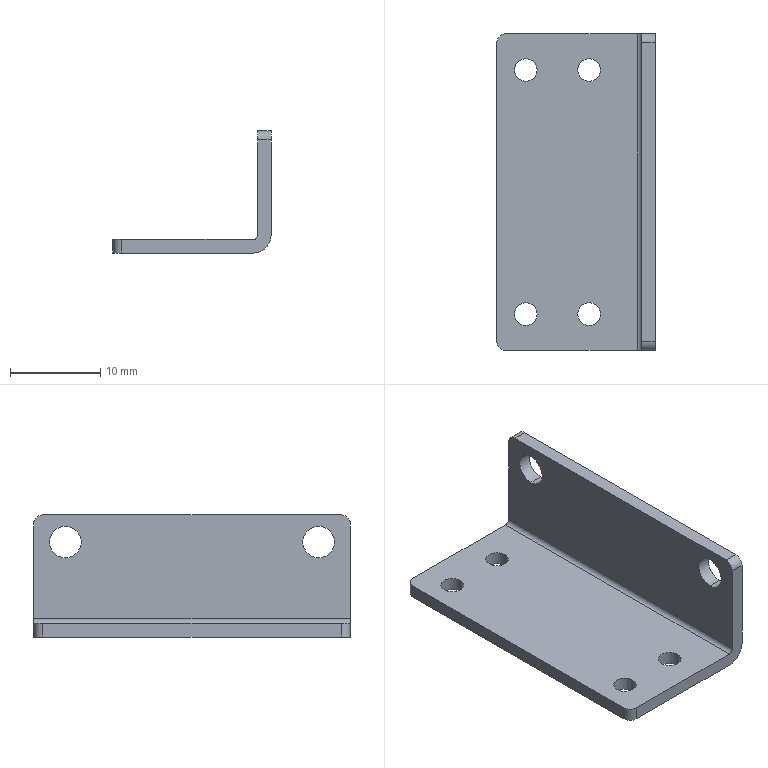Part | SolidWorks | features BaseBody 1 | 1 solid | 26 faces | box 17.5 x 35 x 13.5 mm | volume 1461 mm3 | cylinder 18 | plane 8 | commonest cylinder face diameters 2.5 x8 2 x4 3.5 x4 1 x1 4 x1
STEP:
#1=CARTESIAN_POINT('',(296.997,233.806,-401.845));
#2=VERTEX_POINT('',#1);
#3=CARTESIAN_POINT('',(294.497,233.806,-401.845));
#4=VERTEX_POINT('',#3);
#5=CARTESIAN_POINT('',(295.747,233.806,-401.845));
#6=DIRECTION('',(0.,0.,-1.));
#7=DIRECTION('',(-1.,0.,0.));
#8=AXIS2_PLACEMENT_3D('',#5,#6,#7);
#9=CIRCLE('',#8,1.25);
#10=EDGE_CURVE('',#2,#4,#9,.T.);
#11=ORIENTED_EDGE('',*,*,#10,.F.);
#12=CARTESIAN_POINT('',(296.997,233.806,-403.345));
#13=VERTEX_POINT('',#12);
#14=CARTESIAN_POINT('',(296.997,233.806,-94.345));
#15=DIRECTION('',(0.,0.,-1.));
#16=VECTOR('',#15,1000.);
#17=LINE('',#14,#16);
#18=EDGE_CURVE('',#2,#13,#17,.T.);
#19=ORIENTED_EDGE('',*,*,#18,.T.);
#20=CARTESIAN_POINT('',(294.497,233.806,-403.345));
#21=VERTEX_POINT('',#20);
#22=CARTESIAN_POINT('',(295.747,233.806,-403.345));
#23=DIRECTION('',(0.,0.,-1.));
#24=DIRECTION('',(-1.,0.,0.));
#25=AXIS2_PLACEMENT_3D('',#22,#23,#24);
#26=CIRCLE('',#25,1.25);
#27=EDGE_CURVE('',#13,#21,#26,.T.);
#28=ORIENTED_EDGE('',*,*,#27,.T.);
#29=CARTESIAN_POINT('',(294.497,233.806,-94.345));
#30=DIRECTION('',(0.,0.,-1.));
#31=VECTOR('',#30,1000.);
#32=LINE('',#29,#31);
#33=EDGE_CURVE('',#4,#21,#32,.T.);
#34=ORIENTED_EDGE('',*,*,#33,.F.);
#35=EDGE_LOOP('',(#11,#19,#28,#34));
#36=FACE_OUTER_BOUND('',#35,.T.);
#37=CARTESIAN_POINT('',(295.747,233.806,-94.345));
#38=DIRECTION('',(0.,0.,-1.));
#39=DIRECTION('',(-1.,0.,0.));
#40=AXIS2_PLACEMENT_3D('',#37,#38,#39);
#41=CYLINDRICAL_SURFACE('',#40,1.25);
#42=ADVANCED_FACE('',(#36),#41,.F.);
#43=CARTESIAN_POINT('',(296.997,206.806,-401.845));
#44=VERTEX_POINT('',#43);
#45=CARTESIAN_POINT('',(294.497,206.806,-401.845));
#46=VERTEX_POINT('',#45);
#47=CARTESIAN_POINT('',(295.747,206.806,-401.845));
#48=DIRECTION('',(0.,0.,-1.));
#49=DIRECTION('',(-1.,0.,0.));
#50=AXIS2_PLACEMENT_3D('',#47,#48,#49);
#51=CIRCLE('',#50,1.25);
#52=EDGE_CURVE('',#44,#46,#51,.T.);
#53=ORIENTED_EDGE('',*,*,#52,.F.);
#54=CARTESIAN_POINT('',(296.997,206.806,-403.345));
#55=VERTEX_POINT('',#54);
#56=CARTESIAN_POINT('',(296.997,206.806,-94.345));
#57=DIRECTION('',(0.,0.,-1.));
#58=VECTOR('',#57,1000.);
#59=LINE('',#56,#58);
#60=EDGE_CURVE('',#44,#55,#59,.T.);
#61=ORIENTED_EDGE('',*,*,#60,.T.);
#62=CARTESIAN_POINT('',(294.497,206.806,-403.345));
#63=VERTEX_POINT('',#62);
#64=CARTESIAN_POINT('',(295.747,206.806,-403.345));
#65=DIRECTION('',(0.,0.,-1.));
#66=DIRECTION('',(-1.,0.,0.));
#67=AXIS2_PLACEMENT_3D('',#64,#65,#66);
#68=CIRCLE('',#67,1.25);
#69=EDGE_CURVE('',#55,#63,#68,.T.);
#70=ORIENTED_EDGE('',*,*,#69,.T.);
#71=CARTESIAN_POINT('',(294.497,206.806,-94.345));
#72=DIRECTION('',(0.,0.,-1.));
#73=VECTOR('',#72,1000.);
#74=LINE('',#71,#73);
#75=EDGE_CURVE('',#46,#63,#74,.T.);
#76=ORIENTED_EDGE('',*,*,#75,.F.);
#77=EDGE_LOOP('',(#53,#61,#70,#76));
#78=FACE_OUTER_BOUND('',#77,.T.);
#79=CARTESIAN_POINT('',(295.747,206.806,-94.345));
#80=DIRECTION('',(0.,0.,-1.));
#81=DIRECTION('',(-1.,0.,0.));
#82=AXIS2_PLACEMENT_3D('',#79,#80,#81);
#83=CYLINDRICAL_SURFACE('',#82,1.25);
#84=ADVANCED_FACE('',(#78),#83,.F.);
#85=CARTESIAN_POINT('',(303.997,233.806,-401.845));
#86=VERTEX_POINT('',#85);
#87=CARTESIAN_POINT('',(301.497,233.806,-401.845));
#88=VERTEX_POINT('',#87);
#89=CARTESIAN_POINT('',(302.747,233.806,-401.845));
#90=DIRECTION('',(0.,0.,-1.));
#91=DIRECTION('',(-1.,0.,0.));
#92=AXIS2_PLACEMENT_3D('',#89,#90,#91);
#93=CIRCLE('',#92,1.25);
#94=EDGE_CURVE('',#86,#88,#93,.T.);
#95=ORIENTED_EDGE('',*,*,#94,.F.);
#96=CARTESIAN_POINT('',(303.997,233.806,-403.345));
#97=VERTEX_POINT('',#96);
#98=CARTESIAN_POINT('',(303.997,233.806,-94.345));
#99=DIRECTION('',(0.,0.,-1.));
#100=VECTOR('',#99,1000.);
#101=LINE('',#98,#100);
#102=EDGE_CURVE('',#86,#97,#101,.T.);
#103=ORIENTED_EDGE('',*,*,#102,.T.);
#104=CARTESIAN_POINT('',(301.497,233.806,-403.345));
#105=VERTEX_POINT('',#104);
#106=CARTESIAN_POINT('',(302.747,233.806,-403.345));
#107=DIRECTION('',(0.,0.,-1.));
#108=DIRECTION('',(-1.,0.,0.));
#109=AXIS2_PLACEMENT_3D('',#106,#107,#108);
#110=CIRCLE('',#109,1.25);
#111=EDGE_CURVE('',#97,#105,#110,.T.);
#112=ORIENTED_EDGE('',*,*,#111,.T.);
#113=CARTESIAN_POINT('',(301.497,233.806,-94.345));
#114=DIRECTION('',(0.,0.,-1.));
#115=VECTOR('',#114,1000.);
#116=LINE('',#113,#115);
#117=EDGE_CURVE('',#88,#105,#116,.T.);
#118=ORIENTED_EDGE('',*,*,#117,.F.);
#119=EDGE_LOOP('',(#95,#103,#112,#118));
#120=FACE_OUTER_BOUND('',#119,.T.);
#121=CARTESIAN_POINT('',(302.747,233.806,-94.345));
#122=DIRECTION('',(0.,0.,-1.));
#123=DIRECTION('',(-1.,0.,0.));
#124=AXIS2_PLACEMENT_3D('',#121,#122,#123);
#125=CYLINDRICAL_SURFACE('',#124,1.25);
#126=ADVANCED_FACE('',(#120),#125,.F.);
#127=CARTESIAN_POINT('',(303.997,206.806,-401.845));
#128=VERTEX_POINT('',#127);
#129=CARTESIAN_POINT('',(301.497,206.806,-401.845));
#130=VERTEX_POINT('',#129);
#131=CARTESIAN_POINT('',(302.747,206.806,-401.845));
#132=DIRECTION('',(0.,0.,-1.));
#133=DIRECTION('',(-1.,0.,0.));
#134=AXIS2_PLACEMENT_3D('',#131,#132,#133);
#135=CIRCLE('',#134,1.25);
#136=EDGE_CURVE('',#128,#130,#135,.T.);
#137=ORIENTED_EDGE('',*,*,#136,.F.);
#138=CARTESIAN_POINT('',(303.997,206.806,-403.345));
#139=VERTEX_POINT('',#138);
#140=CARTESIAN_POINT('',(303.997,206.806,-94.345));
#141=DIRECTION('',(0.,0.,-1.));
#142=VECTOR('',#141,1000.);
#143=LINE('',#140,#142);
#144=EDGE_CURVE('',#128,#139,#143,.T.);
#145=ORIENTED_EDGE('',*,*,#144,.T.);
#146=CARTESIAN_POINT('',(301.497,206.806,-403.345));
#147=VERTEX_POINT('',#146);
#148=CARTESIAN_POINT('',(302.747,206.806,-403.345));
#149=DIRECTION('',(0.,0.,-1.));
#150=DIRECTION('',(-1.,0.,0.));
#151=AXIS2_PLACEMENT_3D('',#148,#149,#150);
#152=CIRCLE('',#151,1.25);
#153=EDGE_CURVE('',#139,#147,#152,.T.);
#154=ORIENTED_EDGE('',*,*,#153,.T.);
#155=CARTESIAN_POINT('',(301.497,206.806,-94.345));
#156=DIRECTION('',(0.,0.,-1.));
#157=VECTOR('',#156,1000.);
#158=LINE('',#155,#157);
#159=EDGE_CURVE('',#130,#147,#158,.T.);
#160=ORIENTED_EDGE('',*,*,#159,.F.);
#161=EDGE_LOOP('',(#137,#145,#154,#160));
#162=FACE_OUTER_BOUND('',#161,.T.);
#163=CARTESIAN_POINT('',(302.747,206.806,-94.345));
#164=DIRECTION('',(0.,0.,-1.));
#165=DIRECTION('',(-1.,0.,0.));
#166=AXIS2_PLACEMENT_3D('',#163,#164,#165);
#167=CYLINDRICAL_SURFACE('',#166,1.25);
#168=ADVANCED_FACE('',(#162),#167,.F.);
#169=CARTESIAN_POINT('',(308.547,234.306,-394.595));
#170=VERTEX_POINT('',#169);
#171=CARTESIAN_POINT('',(308.547,234.306,-391.095));
#172=VERTEX_POINT('',#171);
#173=CARTESIAN_POINT('',(308.547,234.306,-392.845));
#174=DIRECTION('',(-1.,0.,0.));
#175=DIRECTION('',(0.,0.,-1.));
#176=AXIS2_PLACEMENT_3D('',#173,#174,#175);
#177=CIRCLE('',#176,1.75);
#178=EDGE_CURVE('',#170,#172,#177,.T.);
#179=ORIENTED_EDGE('',*,*,#178,.T.);
#180=CARTESIAN_POINT('',(310.047,234.306,-391.095));
#181=VERTEX_POINT('',#180);
#182=CARTESIAN_POINT('',(7.247,234.306,-391.095));
#183=DIRECTION('',(1.,0.,0.));
#184=VECTOR('',#183,1000.);
#185=LINE('',#182,#184);
#186=EDGE_CURVE('',#172,#181,#185,.T.);
#187=ORIENTED_EDGE('',*,*,#186,.T.);
#188=CARTESIAN_POINT('',(310.047,234.306,-394.595));
#189=VERTEX_POINT('',#188);
#190=CARTESIAN_POINT('',(310.047,234.306,-392.845));
#191=DIRECTION('',(1.,0.,0.));
#192=DIRECTION('',(0.,0.,-1.));
#193=AXIS2_PLACEMENT_3D('',#190,#191,#192);
#194=CIRCLE('',#193,1.75);
#195=EDGE_CURVE('',#181,#189,#194,.T.);
#196=ORIENTED_EDGE('',*,*,#195,.T.);
#197=CARTESIAN_POINT('',(7.247,234.306,-394.595));
#198=DIRECTION('',(1.,0.,0.));
#199=VECTOR('',#198,1000.);
#200=LINE('',#197,#199);
#201=EDGE_CURVE('',#170,#189,#200,.T.);
#202=ORIENTED_EDGE('',*,*,#201,.F.);
#203=EDGE_LOOP('',(#179,#187,#196,#202));
#204=FACE_OUTER_BOUND('',#203,.T.);
#205=CARTESIAN_POINT('',(7.247,234.306,-392.845));
#206=DIRECTION('',(1.,0.,0.));
#207=DIRECTION('',(0.,0.,-1.));
#208=AXIS2_PLACEMENT_3D('',#205,#206,#207);
#209=CYLINDRICAL_SURFACE('',#208,1.75);
#210=ADVANCED_FACE('',(#204),#209,.F.);
#211=CARTESIAN_POINT('',(308.547,206.306,-394.595));
#212=VERTEX_POINT('',#211);
#213=CARTESIAN_POINT('',(308.547,206.306,-391.095));
#214=VERTEX_POINT('',#213);
#215=CARTESIAN_POINT('',(308.547,206.306,-392.845));
#216=DIRECTION('',(-1.,0.,0.));
#217=DIRECTION('',(0.,0.,-1.));
#218=AXIS2_PLACEMENT_3D('',#215,#216,#217);
#219=CIRCLE('',#218,1.75);
#220=EDGE_CURVE('',#212,#214,#219,.T.);
#221=ORIENTED_EDGE('',*,*,#220,.T.);
#222=CARTESIAN_POINT('',(310.047,206.306,-391.095));
#223=VERTEX_POINT('',#222);
#224=CARTESIAN_POINT('',(7.247,206.306,-391.095));
#225=DIRECTION('',(1.,0.,0.));
#226=VECTOR('',#225,1000.);
#227=LINE('',#224,#226);
#228=EDGE_CURVE('',#214,#223,#227,.T.);
#229=ORIENTED_EDGE('',*,*,#228,.T.);
#230=CARTESIAN_POINT('',(310.047,206.306,-394.595));
#231=VERTEX_POINT('',#230);
#232=CARTESIAN_POINT('',(310.047,206.306,-392.845));
#233=DIRECTION('',(1.,0.,0.));
#234=DIRECTION('',(0.,0.,-1.));
#235=AXIS2_PLACEMENT_3D('',#232,#233,#234);
#236=CIRCLE('',#235,1.75);
#237=EDGE_CURVE('',#223,#231,#236,.T.);
#238=ORIENTED_EDGE('',*,*,#237,.T.);
#239=CARTESIAN_POINT('',(7.247,206.306,-394.595));
#240=DIRECTION('',(1.,0.,0.));
#241=VECTOR('',#240,1000.);
#242=LINE('',#239,#241);
#243=EDGE_CURVE('',#212,#231,#242,.T.);
#244=ORIENTED_EDGE('',*,*,#243,.F.);
#245=EDGE_LOOP('',(#221,#229,#238,#244));
#246=FACE_OUTER_BOUND('',#245,.T.);
#247=CARTESIAN_POINT('',(7.247,206.306,-392.845));
#248=DIRECTION('',(1.,0.,0.));
#249=DIRECTION('',(0.,0.,-1.));
#250=AXIS2_PLACEMENT_3D('',#247,#248,#249);
#251=CYLINDRICAL_SURFACE('',#250,1.75);
#252=ADVANCED_FACE('',(#246),#251,.F.);
#253=CARTESIAN_POINT('',(295.747,233.806,-403.345));
#254=DIRECTION('',(0.,0.,-1.));
#255=DIRECTION('',(-1.,0.,0.));
#256=AXIS2_PLACEMENT_3D('',#253,#254,#255);
#257=CIRCLE('',#256,1.25);
#258=EDGE_CURVE('',#21,#13,#257,.T.);
#259=ORIENTED_EDGE('',*,*,#258,.F.);
#260=ORIENTED_EDGE('',*,*,#27,.F.);
#261=EDGE_LOOP('',(#259,#260));
#262=FACE_BOUND('',#261,.T.);
#263=CARTESIAN_POINT('',(295.747,206.806,-403.345));
#264=DIRECTION('',(0.,0.,-1.));
#265=DIRECTION('',(-1.,0.,0.));
#266=AXIS2_PLACEMENT_3D('',#263,#264,#265);
#267=CIRCLE('',#266,1.25);
#268=EDGE_CURVE('',#63,#55,#267,.T.);
#269=ORIENTED_EDGE('',*,*,#268,.F.);
#270=ORIENTED_EDGE('',*,*,#69,.F.);
#271=EDGE_LOOP('',(#269,#270));
#272=FACE_BOUND('',#271,.T.);
#273=CARTESIAN_POINT('',(302.747,233.806,-403.345));
#274=DIRECTION('',(0.,0.,-1.));
#275=DIRECTION('',(-1.,0.,0.));
#276=AXIS2_PLACEMENT_3D('',#273,#274,#275);
#277=CIRCLE('',#276,1.25);
#278=EDGE_CURVE('',#105,#97,#277,.T.);
#279=ORIENTED_EDGE('',*,*,#278,.F.);
#280=ORIENTED_EDGE('',*,*,#111,.F.);
#281=EDGE_LOOP('',(#279,#280));
#282=FACE_BOUND('',#281,.T.);
#283=CARTESIAN_POINT('',(302.747,206.806,-403.345));
#284=DIRECTION('',(0.,0.,-1.));
#285=DIRECTION('',(-1.,0.,0.));
#286=AXIS2_PLACEMENT_3D('',#283,#284,#285);
#287=CIRCLE('',#286,1.25);
#288=EDGE_CURVE('',#147,#139,#287,.T.);
#289=ORIENTED_EDGE('',*,*,#288,.F.);
#290=ORIENTED_EDGE('',*,*,#153,.F.);
#291=EDGE_LOOP('',(#289,#290));
#292=FACE_BOUND('',#291,.T.);
#293=CARTESIAN_POINT('',(292.547,236.806,-403.345));
#294=VERTEX_POINT('',#293);
#295=CARTESIAN_POINT('',(292.547,203.806,-403.345));
#296=VERTEX_POINT('',#295);
#297=CARTESIAN_POINT('',(292.547,237.806,-403.345));
#298=DIRECTION('',(0.,-1.,0.));
#299=VECTOR('',#298,1000.);
#300=LINE('',#297,#299);
#301=EDGE_CURVE('',#294,#296,#300,.T.);
#302=ORIENTED_EDGE('',*,*,#301,.F.);
#303=CARTESIAN_POINT('',(293.547,237.806,-403.345));
#304=VERTEX_POINT('',#303);
#305=CARTESIAN_POINT('',(293.547,236.806,-403.345));
#306=DIRECTION('',(0.,0.,1.));
#307=DIRECTION('',(-1.,0.,0.));
#308=AXIS2_PLACEMENT_3D('',#305,#306,#307);
#309=CIRCLE('',#308,1.);
#310=EDGE_CURVE('',#304,#294,#309,.T.);
#311=ORIENTED_EDGE('',*,*,#310,.F.);
#312=CARTESIAN_POINT('',(308.047,237.806,-403.345));
#313=VERTEX_POINT('',#312);
#314=CARTESIAN_POINT('',(308.047,237.806,-403.345));
#315=DIRECTION('',(-1.,0.,0.));
#316=VECTOR('',#315,1000.);
#317=LINE('',#314,#316);
#318=EDGE_CURVE('',#313,#304,#317,.T.);
#319=ORIENTED_EDGE('',*,*,#318,.F.);
#320=CARTESIAN_POINT('',(308.047,202.806,-403.345));
#321=VERTEX_POINT('',#320);
#322=CARTESIAN_POINT('',(308.047,237.806,-403.345));
#323=DIRECTION('',(0.,1.,0.));
#324=VECTOR('',#323,1000.);
#325=LINE('',#322,#324);
#326=EDGE_CURVE('',#321,#313,#325,.T.);
#327=ORIENTED_EDGE('',*,*,#326,.F.);
#328=CARTESIAN_POINT('',(293.547,202.806,-403.345));
#329=VERTEX_POINT('',#328);
#330=CARTESIAN_POINT('',(308.047,202.806,-403.345));
#331=DIRECTION('',(1.,0.,0.));
#332=VECTOR('',#331,1000.);
#333=LINE('',#330,#332);
#334=EDGE_CURVE('',#329,#321,#333,.T.);
#335=ORIENTED_EDGE('',*,*,#334,.F.);
#336=CARTESIAN_POINT('',(293.547,203.806,-403.345));
#337=DIRECTION('',(0.,0.,1.));
#338=DIRECTION('',(1.,0.,0.));
#339=AXIS2_PLACEMENT_3D('',#336,#337,#338);
#340=CIRCLE('',#339,1.);
#341=EDGE_CURVE('',#296,#329,#340,.T.);
#342=ORIENTED_EDGE('',*,*,#341,.F.);
#343=EDGE_LOOP('',(#302,#311,#319,#327,#335,#342));
#344=FACE_OUTER_BOUND('',#343,.T.);
#345=CARTESIAN_POINT('',(308.047,237.806,-403.345));
#346=DIRECTION('',(0.,0.,1.));
#347=DIRECTION('',(1.,0.,0.));
#348=AXIS2_PLACEMENT_3D('',#345,#346,#347);
#349=PLANE('',#348);
#350=ADVANCED_FACE('',(#262,#272,#282,#292,#344),#349,.F.);
#351=ORIENTED_EDGE('',*,*,#18,.F.);
#352=CARTESIAN_POINT('',(295.747,233.806,-401.845));
#353=DIRECTION('',(0.,0.,-1.));
#354=DIRECTION('',(-1.,0.,0.));
#355=AXIS2_PLACEMENT_3D('',#352,#353,#354);
#356=CIRCLE('',#355,1.25);
#357=EDGE_CURVE('',#4,#2,#356,.T.);
#358=ORIENTED_EDGE('',*,*,#357,.F.);
#359=ORIENTED_EDGE('',*,*,#33,.T.);
#360=ORIENTED_EDGE('',*,*,#258,.T.);
#361=EDGE_LOOP('',(#351,#358,#359,#360));
#362=FACE_OUTER_BOUND('',#361,.T.);
#363=CARTESIAN_POINT('',(295.747,233.806,-94.345));
#364=DIRECTION('',(0.,0.,-1.));
#365=DIRECTION('',(-1.,0.,0.));
#366=AXIS2_PLACEMENT_3D('',#363,#364,#365);
#367=CYLINDRICAL_SURFACE('',#366,1.25);
#368=ADVANCED_FACE('',(#362),#367,.F.);
#369=ORIENTED_EDGE('',*,*,#60,.F.);
#370=CARTESIAN_POINT('',(295.747,206.806,-401.845));
#371=DIRECTION('',(0.,0.,-1.));
#372=DIRECTION('',(-1.,0.,0.));
#373=AXIS2_PLACEMENT_3D('',#370,#371,#372);
#374=CIRCLE('',#373,1.25);
#375=EDGE_CURVE('',#46,#44,#374,.T.);
#376=ORIENTED_EDGE('',*,*,#375,.F.);
#377=ORIENTED_EDGE('',*,*,#75,.T.);
#378=ORIENTED_EDGE('',*,*,#268,.T.);
#379=EDGE_LOOP('',(#369,#376,#377,#378));
#380=FACE_OUTER_BOUND('',#379,.T.);
#381=CARTESIAN_POINT('',(295.747,206.806,-94.345));
#382=DIRECTION('',(0.,0.,-1.));
#383=DIRECTION('',(-1.,0.,0.));
#384=AXIS2_PLACEMENT_3D('',#381,#382,#383);
#385=CYLINDRICAL_SURFACE('',#384,1.25);
#386=ADVANCED_FACE('',(#380),#385,.F.);
#387=ORIENTED_EDGE('',*,*,#102,.F.);
#388=CARTESIAN_POINT('',(302.747,233.806,-401.845));
#389=DIRECTION('',(0.,0.,-1.));
#390=DIRECTION('',(-1.,0.,0.));
#391=AXIS2_PLACEMENT_3D('',#388,#389,#390);
#392=CIRCLE('',#391,1.25);
#393=EDGE_CURVE('',#88,#86,#392,.T.);
#394=ORIENTED_EDGE('',*,*,#393,.F.);
#395=ORIENTED_EDGE('',*,*,#117,.T.);
#396=ORIENTED_EDGE('',*,*,#278,.T.);
#397=EDGE_LOOP('',(#387,#394,#395,#396));
#398=FACE_OUTER_BOUND('',#397,.T.);
#399=CARTESIAN_POINT('',(302.747,233.806,-94.345));
#400=DIRECTION('',(0.,0.,-1.));
#401=DIRECTION('',(-1.,0.,0.));
#402=AXIS2_PLACEMENT_3D('',#399,#400,#401);
#403=CYLINDRICAL_SURFACE('',#402,1.25);
#404=ADVANCED_FACE('',(#398),#403,.F.);
#405=ORIENTED_EDGE('',*,*,#144,.F.);
#406=CARTESIAN_POINT('',(302.747,206.806,-401.845));
#407=DIRECTION('',(0.,0.,-1.));
#408=DIRECTION('',(-1.,0.,0.));
#409=AXIS2_PLACEMENT_3D('',#406,#407,#408);
#410=CIRCLE('',#409,1.25);
#411=EDGE_CURVE('',#130,#128,#410,.T.);
#412=ORIENTED_EDGE('',*,*,#411,.F.);
#413=ORIENTED_EDGE('',*,*,#159,.T.);
#414=ORIENTED_EDGE('',*,*,#288,.T.);
#415=EDGE_LOOP('',(#405,#412,#413,#414));
#416=FACE_OUTER_BOUND('',#415,.T.);
#417=CARTESIAN_POINT('',(302.747,206.806,-94.345));
#418=DIRECTION('',(0.,0.,-1.));
#419=DIRECTION('',(-1.,0.,0.));
#420=AXIS2_PLACEMENT_3D('',#417,#418,#419);
#421=CYLINDRICAL_SURFACE('',#420,1.25);
#422=ADVANCED_FACE('',(#416),#421,.F.);
#423=CARTESIAN_POINT('',(292.547,203.806,-401.845));
#424=VERTEX_POINT('',#423);
#425=CARTESIAN_POINT('',(292.547,203.806,-403.345));
#426=DIRECTION('',(0.,0.,-1.));
#427=VECTOR('',#426,1000.);
#428=LINE('',#425,#427);
#429=EDGE_CURVE('',#424,#296,#428,.T.);
#430=ORIENTED_EDGE('',*,*,#429,.T.);
#431=ORIENTED_EDGE('',*,*,#341,.T.);
#432=CARTESIAN_POINT('',(293.547,202.806,-401.845));
#433=VERTEX_POINT('',#432);
#434=CARTESIAN_POINT('',(293.547,202.806,-403.345));
#435=DIRECTION('',(0.,0.,1.));
#436=VECTOR('',#435,1000.);
#437=LINE('',#434,#436);
#438=EDGE_CURVE('',#329,#433,#437,.T.);
#439=ORIENTED_EDGE('',*,*,#438,.T.);
#440=CARTESIAN_POINT('',(293.547,203.806,-401.845));
#441=DIRECTION('',(0.,0.,-1.));
#442=DIRECTION('',(1.,0.,0.));
#443=AXIS2_PLACEMENT_3D('',#440,#441,#442);
#444=CIRCLE('',#443,1.);
#445=EDGE_CURVE('',#433,#424,#444,.T.);
#446=ORIENTED_EDGE('',*,*,#445,.T.);
#447=EDGE_LOOP('',(#430,#431,#439,#446));
#448=FACE_OUTER_BOUND('',#447,.T.);
#449=CARTESIAN_POINT('',(293.547,203.806,-403.345));
#450=DIRECTION('',(0.,0.,1.));
#451=DIRECTION('',(1.,0.,0.));
#452=AXIS2_PLACEMENT_3D('',#449,#450,#451);
#453=CYLINDRICAL_SURFACE('',#452,1.);
#454=ADVANCED_FACE('',(#448),#453,.T.);
#455=CARTESIAN_POINT('',(292.547,236.806,-401.845));
#456=VERTEX_POINT('',#455);
#457=CARTESIAN_POINT('',(292.547,237.806,-401.845));
#458=DIRECTION('',(0.,-1.,0.));
#459=VECTOR('',#458,1000.);
#460=LINE('',#457,#459);
#461=EDGE_CURVE('',#456,#424,#460,.T.);
#462=ORIENTED_EDGE('',*,*,#461,.F.);
#463=CARTESIAN_POINT('',(292.547,236.806,-403.345));
#464=DIRECTION('',(0.,0.,1.));
#465=VECTOR('',#464,1000.);
#466=LINE('',#463,#465);
#467=EDGE_CURVE('',#294,#456,#466,.T.);
#468=ORIENTED_EDGE('',*,*,#467,.F.);
#469=ORIENTED_EDGE('',*,*,#301,.T.);
#470=ORIENTED_EDGE('',*,*,#429,.F.);
#471=EDGE_LOOP('',(#462,#468,#469,#470));
#472=FACE_OUTER_BOUND('',#471,.T.);
#473=CARTESIAN_POINT('',(292.547,237.806,-403.345));
#474=DIRECTION('',(1.,0.,0.));
#475=DIRECTION('',(0.,0.,-1.));
#476=AXIS2_PLACEMENT_3D('',#473,#474,#475);
#477=PLANE('',#476);
#478=ADVANCED_FACE('',(#472),#477,.F.);
#479=CARTESIAN_POINT('',(293.547,237.806,-401.845));
#480=VERTEX_POINT('',#479);
#481=CARTESIAN_POINT('',(293.547,237.806,-401.345));
#482=DIRECTION('',(0.,0.,-1.));
#483=VECTOR('',#482,1000.);
#484=LINE('',#481,#483);
#485=EDGE_CURVE('',#480,#304,#484,.T.);
#486=ORIENTED_EDGE('',*,*,#485,.T.);
#487=ORIENTED_EDGE('',*,*,#310,.T.);
#488=ORIENTED_EDGE('',*,*,#467,.T.);
#489=CARTESIAN_POINT('',(293.547,236.806,-401.845));
#490=DIRECTION('',(0.,0.,-1.));
#491=DIRECTION('',(-1.,0.,0.));
#492=AXIS2_PLACEMENT_3D('',#489,#490,#491);
#493=CIRCLE('',#492,1.);
#494=EDGE_CURVE('',#456,#480,#493,.T.);
#495=ORIENTED_EDGE('',*,*,#494,.T.);
#496=EDGE_LOOP('',(#486,#487,#488,#495));
#497=FACE_OUTER_BOUND('',#496,.T.);
#498=CARTESIAN_POINT('',(293.547,236.806,-401.345));
#499=DIRECTION('',(0.,0.,-1.));
#500=DIRECTION('',(-1.,0.,0.));
#501=AXIS2_PLACEMENT_3D('',#498,#499,#500);
#502=CYLINDRICAL_SURFACE('',#501,1.);
#503=ADVANCED_FACE('',(#497),#502,.T.);
#504=CARTESIAN_POINT('',(308.047,237.806,-401.845));
#505=VERTEX_POINT('',#504);
#506=CARTESIAN_POINT('',(308.547,237.806,-401.345));
#507=VERTEX_POINT('',#506);
#508=CARTESIAN_POINT('',(308.047,237.806,-401.345));
#509=DIRECTION('',(0.,-1.,0.));
#510=DIRECTION('',(0.,0.,-1.));
#511=AXIS2_PLACEMENT_3D('',#508,#509,#510);
#512=CIRCLE('',#511,0.5);
#513=EDGE_CURVE('',#505,#507,#512,.T.);
#514=ORIENTED_EDGE('',*,*,#513,.T.);
#515=CARTESIAN_POINT('',(308.547,237.806,-390.845));
#516=VERTEX_POINT('',#515);
#517=CARTESIAN_POINT('',(308.547,237.806,-401.345));
#518=DIRECTION('',(0.,0.,1.));
#519=VECTOR('',#518,1000.);
#520=LINE('',#517,#519);
#521=EDGE_CURVE('',#507,#516,#520,.T.);
#522=ORIENTED_EDGE('',*,*,#521,.T.);
#523=CARTESIAN_POINT('',(310.047,237.806,-390.845));
#524=VERTEX_POINT('',#523);
#525=CARTESIAN_POINT('',(308.047,237.806,-390.845));
#526=DIRECTION('',(1.,0.,0.));
#527=VECTOR('',#526,1000.);
#528=LINE('',#525,#527);
#529=EDGE_CURVE('',#516,#524,#528,.T.);
#530=ORIENTED_EDGE('',*,*,#529,.T.);
#531=CARTESIAN_POINT('',(310.047,237.806,-401.345));
#532=VERTEX_POINT('',#531);
#533=CARTESIAN_POINT('',(310.047,237.806,-401.345));
#534=DIRECTION('',(0.,0.,-1.));
#535=VECTOR('',#534,1000.);
#536=LINE('',#533,#535);
#537=EDGE_CURVE('',#524,#532,#536,.T.);
#538=ORIENTED_EDGE('',*,*,#537,.T.);
#539=CARTESIAN_POINT('',(308.047,237.806,-401.345));
#540=DIRECTION('',(0.,1.,0.));
#541=DIRECTION('',(0.,0.,-1.));
#542=AXIS2_PLACEMENT_3D('',#539,#540,#541);
#543=CIRCLE('',#542,2.);
#544=EDGE_CURVE('',#532,#313,#543,.T.);
#545=ORIENTED_EDGE('',*,*,#544,.T.);
#546=ORIENTED_EDGE('',*,*,#318,.T.);
#547=ORIENTED_EDGE('',*,*,#485,.F.);
#548=CARTESIAN_POINT('',(308.047,237.806,-401.845));
#549=DIRECTION('',(1.,0.,0.));
#550=VECTOR('',#549,1000.);
#551=LINE('',#548,#550);
#552=EDGE_CURVE('',#480,#505,#551,.T.);
#553=ORIENTED_EDGE('',*,*,#552,.T.);
#554=EDGE_LOOP('',(#514,#522,#530,#538,#545,#546,#547,#553));
#555=FACE_OUTER_BOUND('',#554,.T.);
#556=CARTESIAN_POINT('',(308.047,237.806,-401.345));
#557=DIRECTION('',(0.,1.,0.));
#558=DIRECTION('',(0.,0.,1.));
#559=AXIS2_PLACEMENT_3D('',#556,#557,#558);
#560=PLANE('',#559);
#561=ADVANCED_FACE('',(#555),#560,.T.);
#562=CARTESIAN_POINT('',(310.047,202.806,-401.345));
#563=VERTEX_POINT('',#562);
#564=CARTESIAN_POINT('',(310.047,237.806,-401.345));
#565=DIRECTION('',(0.,-1.,0.));
#566=VECTOR('',#565,1000.);
#567=LINE('',#564,#566);
#568=EDGE_CURVE('',#532,#563,#567,.T.);
#569=ORIENTED_EDGE('',*,*,#568,.T.);
#570=CARTESIAN_POINT('',(308.047,202.806,-401.345));
#571=DIRECTION('',(0.,1.,0.));
#572=DIRECTION('',(0.,0.,-1.));
#573=AXIS2_PLACEMENT_3D('',#570,#571,#572);
#574=CIRCLE('',#573,2.);
#575=EDGE_CURVE('',#563,#321,#574,.T.);
#576=ORIENTED_EDGE('',*,*,#575,.T.);
#577=ORIENTED_EDGE('',*,*,#326,.T.);
#578=ORIENTED_EDGE('',*,*,#544,.F.);
#579=EDGE_LOOP('',(#569,#576,#577,#578));
#580=FACE_OUTER_BOUND('',#579,.T.);
#581=CARTESIAN_POINT('',(308.047,237.806,-401.345));
#582=DIRECTION('',(0.,-1.,0.));
#583=DIRECTION('',(0.,0.,-1.));
#584=AXIS2_PLACEMENT_3D('',#581,#582,#583);
#585=CYLINDRICAL_SURFACE('',#584,2.);
#586=ADVANCED_FACE('',(#580),#585,.T.);
#587=ORIENTED_EDGE('',*,*,#334,.T.);
#588=ORIENTED_EDGE('',*,*,#575,.F.);
#589=CARTESIAN_POINT('',(310.047,202.806,-390.845));
#590=VERTEX_POINT('',#589);
#591=CARTESIAN_POINT('',(310.047,202.806,-401.345));
#592=DIRECTION('',(0.,0.,-1.));
#593=VECTOR('',#592,1000.);
#594=LINE('',#591,#593);
#595=EDGE_CURVE('',#590,#563,#594,.T.);
#596=ORIENTED_EDGE('',*,*,#595,.F.);
#597=CARTESIAN_POINT('',(308.547,202.806,-390.845));
#598=VERTEX_POINT('',#597);
#599=CARTESIAN_POINT('',(308.047,202.806,-390.845));
#600=DIRECTION('',(1.,0.,0.));
#601=VECTOR('',#600,1000.);
#602=LINE('',#599,#601);
#603=EDGE_CURVE('',#598,#590,#602,.T.);
#604=ORIENTED_EDGE('',*,*,#603,.F.);
#605=CARTESIAN_POINT('',(308.547,202.806,-401.345));
#606=VERTEX_POINT('',#605);
#607=CARTESIAN_POINT('',(308.547,202.806,-401.345));
#608=DIRECTION('',(0.,0.,1.));
#609=VECTOR('',#608,1000.);
#610=LINE('',#607,#609);
#611=EDGE_CURVE('',#606,#598,#610,.T.);
#612=ORIENTED_EDGE('',*,*,#611,.F.);
#613=CARTESIAN_POINT('',(308.047,202.806,-401.845));
#614=VERTEX_POINT('',#613);
#615=CARTESIAN_POINT('',(308.047,202.806,-401.345));
#616=DIRECTION('',(0.,-1.,0.));
#617=DIRECTION('',(0.,0.,-1.));
#618=AXIS2_PLACEMENT_3D('',#615,#616,#617);
#619=CIRCLE('',#618,0.5);
#620=EDGE_CURVE('',#614,#606,#619,.T.);
#621=ORIENTED_EDGE('',*,*,#620,.F.);
#622=CARTESIAN_POINT('',(308.047,202.806,-401.845));
#623=DIRECTION('',(1.,0.,0.));
#624=VECTOR('',#623,1000.);
#625=LINE('',#622,#624);
#626=EDGE_CURVE('',#433,#614,#625,.T.);
#627=ORIENTED_EDGE('',*,*,#626,.F.);
#628=ORIENTED_EDGE('',*,*,#438,.F.);
#629=EDGE_LOOP('',(#587,#588,#596,#604,#612,#621,#627,#628));
#630=FACE_OUTER_BOUND('',#629,.T.);
#631=CARTESIAN_POINT('',(308.047,202.806,-401.345));
#632=DIRECTION('',(0.,1.,0.));
#633=DIRECTION('',(0.,0.,1.));
#634=AXIS2_PLACEMENT_3D('',#631,#632,#633);
#635=PLANE('',#634);
#636=ADVANCED_FACE('',(#630),#635,.F.);
#637=ORIENTED_EDGE('',*,*,#357,.T.);
#638=ORIENTED_EDGE('',*,*,#10,.T.);
#639=EDGE_LOOP('',(#637,#638));
#640=FACE_BOUND('',#639,.T.);
#641=ORIENTED_EDGE('',*,*,#375,.T.);
#642=ORIENTED_EDGE('',*,*,#52,.T.);
#643=EDGE_LOOP('',(#641,#642));
#644=FACE_BOUND('',#643,.T.);
#645=ORIENTED_EDGE('',*,*,#393,.T.);
#646=ORIENTED_EDGE('',*,*,#94,.T.);
#647=EDGE_LOOP('',(#645,#646));
#648=FACE_BOUND('',#647,.T.);
#649=ORIENTED_EDGE('',*,*,#411,.T.);
#650=ORIENTED_EDGE('',*,*,#136,.T.);
#651=EDGE_LOOP('',(#649,#650));
#652=FACE_BOUND('',#651,.T.);
#653=ORIENTED_EDGE('',*,*,#626,.T.);
#654=CARTESIAN_POINT('',(308.047,237.806,-401.845));
#655=DIRECTION('',(0.,-1.,0.));
#656=VECTOR('',#655,1000.);
#657=LINE('',#654,#656);
#658=EDGE_CURVE('',#505,#614,#657,.T.);
#659=ORIENTED_EDGE('',*,*,#658,.F.);
#660=ORIENTED_EDGE('',*,*,#552,.F.);
#661=ORIENTED_EDGE('',*,*,#494,.F.);
#662=ORIENTED_EDGE('',*,*,#461,.T.);
#663=ORIENTED_EDGE('',*,*,#445,.F.);
#664=EDGE_LOOP('',(#653,#659,#660,#661,#662,#663));
#665=FACE_OUTER_BOUND('',#664,.T.);
#666=CARTESIAN_POINT('',(292.547,237.806,-401.845));
#667=DIRECTION('',(0.,0.,-1.));
#668=DIRECTION('',(-1.,0.,0.));
#669=AXIS2_PLACEMENT_3D('',#666,#667,#668);
#670=PLANE('',#669);
#671=ADVANCED_FACE('',(#640,#644,#648,#652,#665),#670,.F.);
#672=ORIENTED_EDGE('',*,*,#178,.F.);
#673=CARTESIAN_POINT('',(308.547,234.306,-392.845));
#674=DIRECTION('',(-1.,0.,0.));
#675=DIRECTION('',(0.,0.,-1.));
#676=AXIS2_PLACEMENT_3D('',#673,#674,#675);
#677=CIRCLE('',#676,1.75);
#678=EDGE_CURVE('',#172,#170,#677,.T.);
#679=ORIENTED_EDGE('',*,*,#678,.F.);
#680=EDGE_LOOP('',(#672,#679));
#681=FACE_BOUND('',#680,.T.);
#682=ORIENTED_EDGE('',*,*,#220,.F.);
#683=CARTESIAN_POINT('',(308.547,206.306,-392.845));
#684=DIRECTION('',(-1.,0.,0.));
#685=DIRECTION('',(0.,0.,-1.));
#686=AXIS2_PLACEMENT_3D('',#683,#684,#685);
#687=CIRCLE('',#686,1.75);
#688=EDGE_CURVE('',#214,#212,#687,.T.);
#689=ORIENTED_EDGE('',*,*,#688,.F.);
#690=EDGE_LOOP('',(#682,#689));
#691=FACE_BOUND('',#690,.T.);
#692=ORIENTED_EDGE('',*,*,#521,.F.);
#693=CARTESIAN_POINT('',(308.547,237.806,-401.345));
#694=DIRECTION('',(0.,1.,0.));
#695=VECTOR('',#694,1000.);
#696=LINE('',#693,#695);
#697=EDGE_CURVE('',#606,#507,#696,.T.);
#698=ORIENTED_EDGE('',*,*,#697,.F.);
#699=ORIENTED_EDGE('',*,*,#611,.T.);
#700=CARTESIAN_POINT('',(308.547,203.806,-389.845));
#701=VERTEX_POINT('',#700);
#702=CARTESIAN_POINT('',(308.547,203.806,-390.845));
#703=DIRECTION('',(1.,0.,0.));
#704=DIRECTION('',(0.,0.,-1.));
#705=AXIS2_PLACEMENT_3D('',#702,#703,#704);
#706=CIRCLE('',#705,1.);
#707=EDGE_CURVE('',#701,#598,#706,.T.);
#708=ORIENTED_EDGE('',*,*,#707,.F.);
#709=CARTESIAN_POINT('',(308.547,236.806,-389.845));
#710=VERTEX_POINT('',#709);
#711=CARTESIAN_POINT('',(308.547,237.806,-389.845));
#712=DIRECTION('',(0.,-1.,0.));
#713=VECTOR('',#712,1000.);
#714=LINE('',#711,#713);
#715=EDGE_CURVE('',#710,#701,#714,.T.);
#716=ORIENTED_EDGE('',*,*,#715,.F.);
#717=CARTESIAN_POINT('',(308.547,236.806,-390.845));
#718=DIRECTION('',(1.,0.,0.));
#719=DIRECTION('',(0.,0.,1.));
#720=AXIS2_PLACEMENT_3D('',#717,#718,#719);
#721=CIRCLE('',#720,1.);
#722=EDGE_CURVE('',#516,#710,#721,.T.);
#723=ORIENTED_EDGE('',*,*,#722,.F.);
#724=EDGE_LOOP('',(#692,#698,#699,#708,#716,#723));
#725=FACE_OUTER_BOUND('',#724,.T.);
#726=CARTESIAN_POINT('',(308.547,237.806,-401.345));
#727=DIRECTION('',(1.,0.,0.));
#728=DIRECTION('',(0.,0.,-1.));
#729=AXIS2_PLACEMENT_3D('',#726,#727,#728);
#730=PLANE('',#729);
#731=ADVANCED_FACE('',(#681,#691,#725),#730,.F.);
#732=ORIENTED_EDGE('',*,*,#513,.F.);
#733=ORIENTED_EDGE('',*,*,#658,.T.);
#734=ORIENTED_EDGE('',*,*,#620,.T.);
#735=ORIENTED_EDGE('',*,*,#697,.T.);
#736=EDGE_LOOP('',(#732,#733,#734,#735));
#737=FACE_OUTER_BOUND('',#736,.T.);
#738=CARTESIAN_POINT('',(308.047,237.806,-401.345));
#739=DIRECTION('',(0.,-1.,0.));
#740=DIRECTION('',(0.,0.,-1.));
#741=AXIS2_PLACEMENT_3D('',#738,#739,#740);
#742=CYLINDRICAL_SURFACE('',#741,0.5);
#743=ADVANCED_FACE('',(#737),#742,.F.);
#744=CARTESIAN_POINT('',(310.047,234.306,-392.845));
#745=DIRECTION('',(1.,0.,0.));
#746=DIRECTION('',(0.,0.,-1.));
#747=AXIS2_PLACEMENT_3D('',#744,#745,#746);
#748=CIRCLE('',#747,1.75);
#749=EDGE_CURVE('',#189,#181,#748,.T.);
#750=ORIENTED_EDGE('',*,*,#749,.F.);
#751=ORIENTED_EDGE('',*,*,#195,.F.);
#752=EDGE_LOOP('',(#750,#751));
#753=FACE_BOUND('',#752,.T.);
#754=CARTESIAN_POINT('',(310.047,206.306,-392.845));
#755=DIRECTION('',(1.,0.,0.));
#756=DIRECTION('',(0.,0.,-1.));
#757=AXIS2_PLACEMENT_3D('',#754,#755,#756);
#758=CIRCLE('',#757,1.75);
#759=EDGE_CURVE('',#231,#223,#758,.T.);
#760=ORIENTED_EDGE('',*,*,#759,.F.);
#761=ORIENTED_EDGE('',*,*,#237,.F.);
#762=EDGE_LOOP('',(#760,#761));
#763=FACE_BOUND('',#762,.T.);
#764=CARTESIAN_POINT('',(310.047,203.806,-389.845));
#765=VERTEX_POINT('',#764);
#766=CARTESIAN_POINT('',(310.047,236.806,-389.845));
#767=VERTEX_POINT('',#766);
#768=CARTESIAN_POINT('',(310.047,237.806,-389.845));
#769=DIRECTION('',(0.,1.,0.));
#770=VECTOR('',#769,1000.);
#771=LINE('',#768,#770);
#772=EDGE_CURVE('',#765,#767,#771,.T.);
#773=ORIENTED_EDGE('',*,*,#772,.F.);
#774=CARTESIAN_POINT('',(310.047,203.806,-390.845));
#775=DIRECTION('',(-1.,0.,0.));
#776=DIRECTION('',(0.,0.,-1.));
#777=AXIS2_PLACEMENT_3D('',#774,#775,#776);
#778=CIRCLE('',#777,1.);
#779=EDGE_CURVE('',#590,#765,#778,.T.);
#780=ORIENTED_EDGE('',*,*,#779,.F.);
#781=ORIENTED_EDGE('',*,*,#595,.T.);
#782=ORIENTED_EDGE('',*,*,#568,.F.);
#783=ORIENTED_EDGE('',*,*,#537,.F.);
#784=CARTESIAN_POINT('',(310.047,236.806,-390.845));
#785=DIRECTION('',(-1.,0.,0.));
#786=DIRECTION('',(0.,0.,1.));
#787=AXIS2_PLACEMENT_3D('',#784,#785,#786);
#788=CIRCLE('',#787,1.);
#789=EDGE_CURVE('',#767,#524,#788,.T.);
#790=ORIENTED_EDGE('',*,*,#789,.F.);
#791=EDGE_LOOP('',(#773,#780,#781,#782,#783,#790));
#792=FACE_OUTER_BOUND('',#791,.T.);
#793=CARTESIAN_POINT('',(310.047,237.806,-389.845));
#794=DIRECTION('',(-1.,0.,0.));
#795=DIRECTION('',(0.,0.,1.));
#796=AXIS2_PLACEMENT_3D('',#793,#794,#795);
#797=PLANE('',#796);
#798=ADVANCED_FACE('',(#753,#763,#792),#797,.F.);
#799=ORIENTED_EDGE('',*,*,#529,.F.);
#800=ORIENTED_EDGE('',*,*,#722,.T.);
#801=CARTESIAN_POINT('',(308.047,236.806,-389.845));
#802=DIRECTION('',(1.,0.,0.));
#803=VECTOR('',#802,1000.);
#804=LINE('',#801,#803);
#805=EDGE_CURVE('',#710,#767,#804,.T.);
#806=ORIENTED_EDGE('',*,*,#805,.T.);
#807=ORIENTED_EDGE('',*,*,#789,.T.);
#808=EDGE_LOOP('',(#799,#800,#806,#807));
#809=FACE_OUTER_BOUND('',#808,.T.);
#810=CARTESIAN_POINT('',(308.047,236.806,-390.845));
#811=DIRECTION('',(-1.,0.,0.));
#812=DIRECTION('',(0.,0.,1.));
#813=AXIS2_PLACEMENT_3D('',#810,#811,#812);
#814=CYLINDRICAL_SURFACE('',#813,1.);
#815=ADVANCED_FACE('',(#809),#814,.T.);
#816=CARTESIAN_POINT('',(308.547,203.806,-389.845));
#817=DIRECTION('',(-1.,0.,0.));
#818=VECTOR('',#817,1000.);
#819=LINE('',#816,#818);
#820=EDGE_CURVE('',#765,#701,#819,.T.);
#821=ORIENTED_EDGE('',*,*,#820,.T.);
#822=ORIENTED_EDGE('',*,*,#707,.T.);
#823=ORIENTED_EDGE('',*,*,#603,.T.);
#824=ORIENTED_EDGE('',*,*,#779,.T.);
#825=EDGE_LOOP('',(#821,#822,#823,#824));
#826=FACE_OUTER_BOUND('',#825,.T.);
#827=CARTESIAN_POINT('',(308.547,203.806,-390.845));
#828=DIRECTION('',(1.,0.,0.));
#829=DIRECTION('',(0.,0.,-1.));
#830=AXIS2_PLACEMENT_3D('',#827,#828,#829);
#831=CYLINDRICAL_SURFACE('',#830,1.);
#832=ADVANCED_FACE('',(#826),#831,.T.);
#833=ORIENTED_EDGE('',*,*,#186,.F.);
#834=ORIENTED_EDGE('',*,*,#678,.T.);
#835=ORIENTED_EDGE('',*,*,#201,.T.);
#836=ORIENTED_EDGE('',*,*,#749,.T.);
#837=EDGE_LOOP('',(#833,#834,#835,#836));
#838=FACE_OUTER_BOUND('',#837,.T.);
#839=CARTESIAN_POINT('',(7.247,234.306,-392.845));
#840=DIRECTION('',(1.,0.,0.));
#841=DIRECTION('',(0.,0.,-1.));
#842=AXIS2_PLACEMENT_3D('',#839,#840,#841);
#843=CYLINDRICAL_SURFACE('',#842,1.75);
#844=ADVANCED_FACE('',(#838),#843,.F.);
#845=ORIENTED_EDGE('',*,*,#228,.F.);
#846=ORIENTED_EDGE('',*,*,#688,.T.);
#847=ORIENTED_EDGE('',*,*,#243,.T.);
#848=ORIENTED_EDGE('',*,*,#759,.T.);
#849=EDGE_LOOP('',(#845,#846,#847,#848));
#850=FACE_OUTER_BOUND('',#849,.T.);
#851=CARTESIAN_POINT('',(7.247,206.306,-392.845));
#852=DIRECTION('',(1.,0.,0.));
#853=DIRECTION('',(0.,0.,-1.));
#854=AXIS2_PLACEMENT_3D('',#851,#852,#853);
#855=CYLINDRICAL_SURFACE('',#854,1.75);
#856=ADVANCED_FACE('',(#850),#855,.F.);
#857=ORIENTED_EDGE('',*,*,#715,.T.);
#858=ORIENTED_EDGE('',*,*,#820,.F.);
#859=ORIENTED_EDGE('',*,*,#772,.T.);
#860=ORIENTED_EDGE('',*,*,#805,.F.);
#861=EDGE_LOOP('',(#857,#858,#859,#860));
#862=FACE_OUTER_BOUND('',#861,.T.);
#863=CARTESIAN_POINT('',(308.547,237.806,-389.845));
#864=DIRECTION('',(0.,0.,-1.));
#865=DIRECTION('',(-1.,0.,0.));
#866=AXIS2_PLACEMENT_3D('',#863,#864,#865);
#867=PLANE('',#866);
#868=ADVANCED_FACE('',(#862),#867,.F.);
#869=CLOSED_SHELL('',(#42,#84,#126,#168,#210,#252,#350,#368,#386,#404,#422,#454,#478,#503,#561,#586,#636,#671,#731,#743,#798,#815,#832,#844,#856,#868));
#870=MANIFOLD_SOLID_BREP('',#869);
#871=CARTESIAN_POINT('',(0.,0.,0.));
#872=DIRECTION('',(0.,0.,1.));
#873=DIRECTION('',(1.,0.,0.));
#874=AXIS2_PLACEMENT_3D('',#871,#872,#873);
#875=(LENGTH_UNIT()NAMED_UNIT(*)SI_UNIT(.MILLI.,.METRE.));
#876=UNCERTAINTY_MEASURE_WITH_UNIT(LENGTH_MEASURE(0.00001),#875,'','');
#877=(NAMED_UNIT(*)PLANE_ANGLE_UNIT()SI_UNIT($,.RADIAN.));
#878=(NAMED_UNIT(*)SI_UNIT($,.STERADIAN.)SOLID_ANGLE_UNIT());
#879=(GEOMETRIC_REPRESENTATION_CONTEXT(3)GLOBAL_UNCERTAINTY_ASSIGNED_CONTEXT((#876))GLOBAL_UNIT_ASSIGNED_CONTEXT((#875,#877,#878))REPRESENTATION_CONTEXT('',''));
#880=ADVANCED_BREP_SHAPE_REPRESENTATION('',(#870,#874),#879);